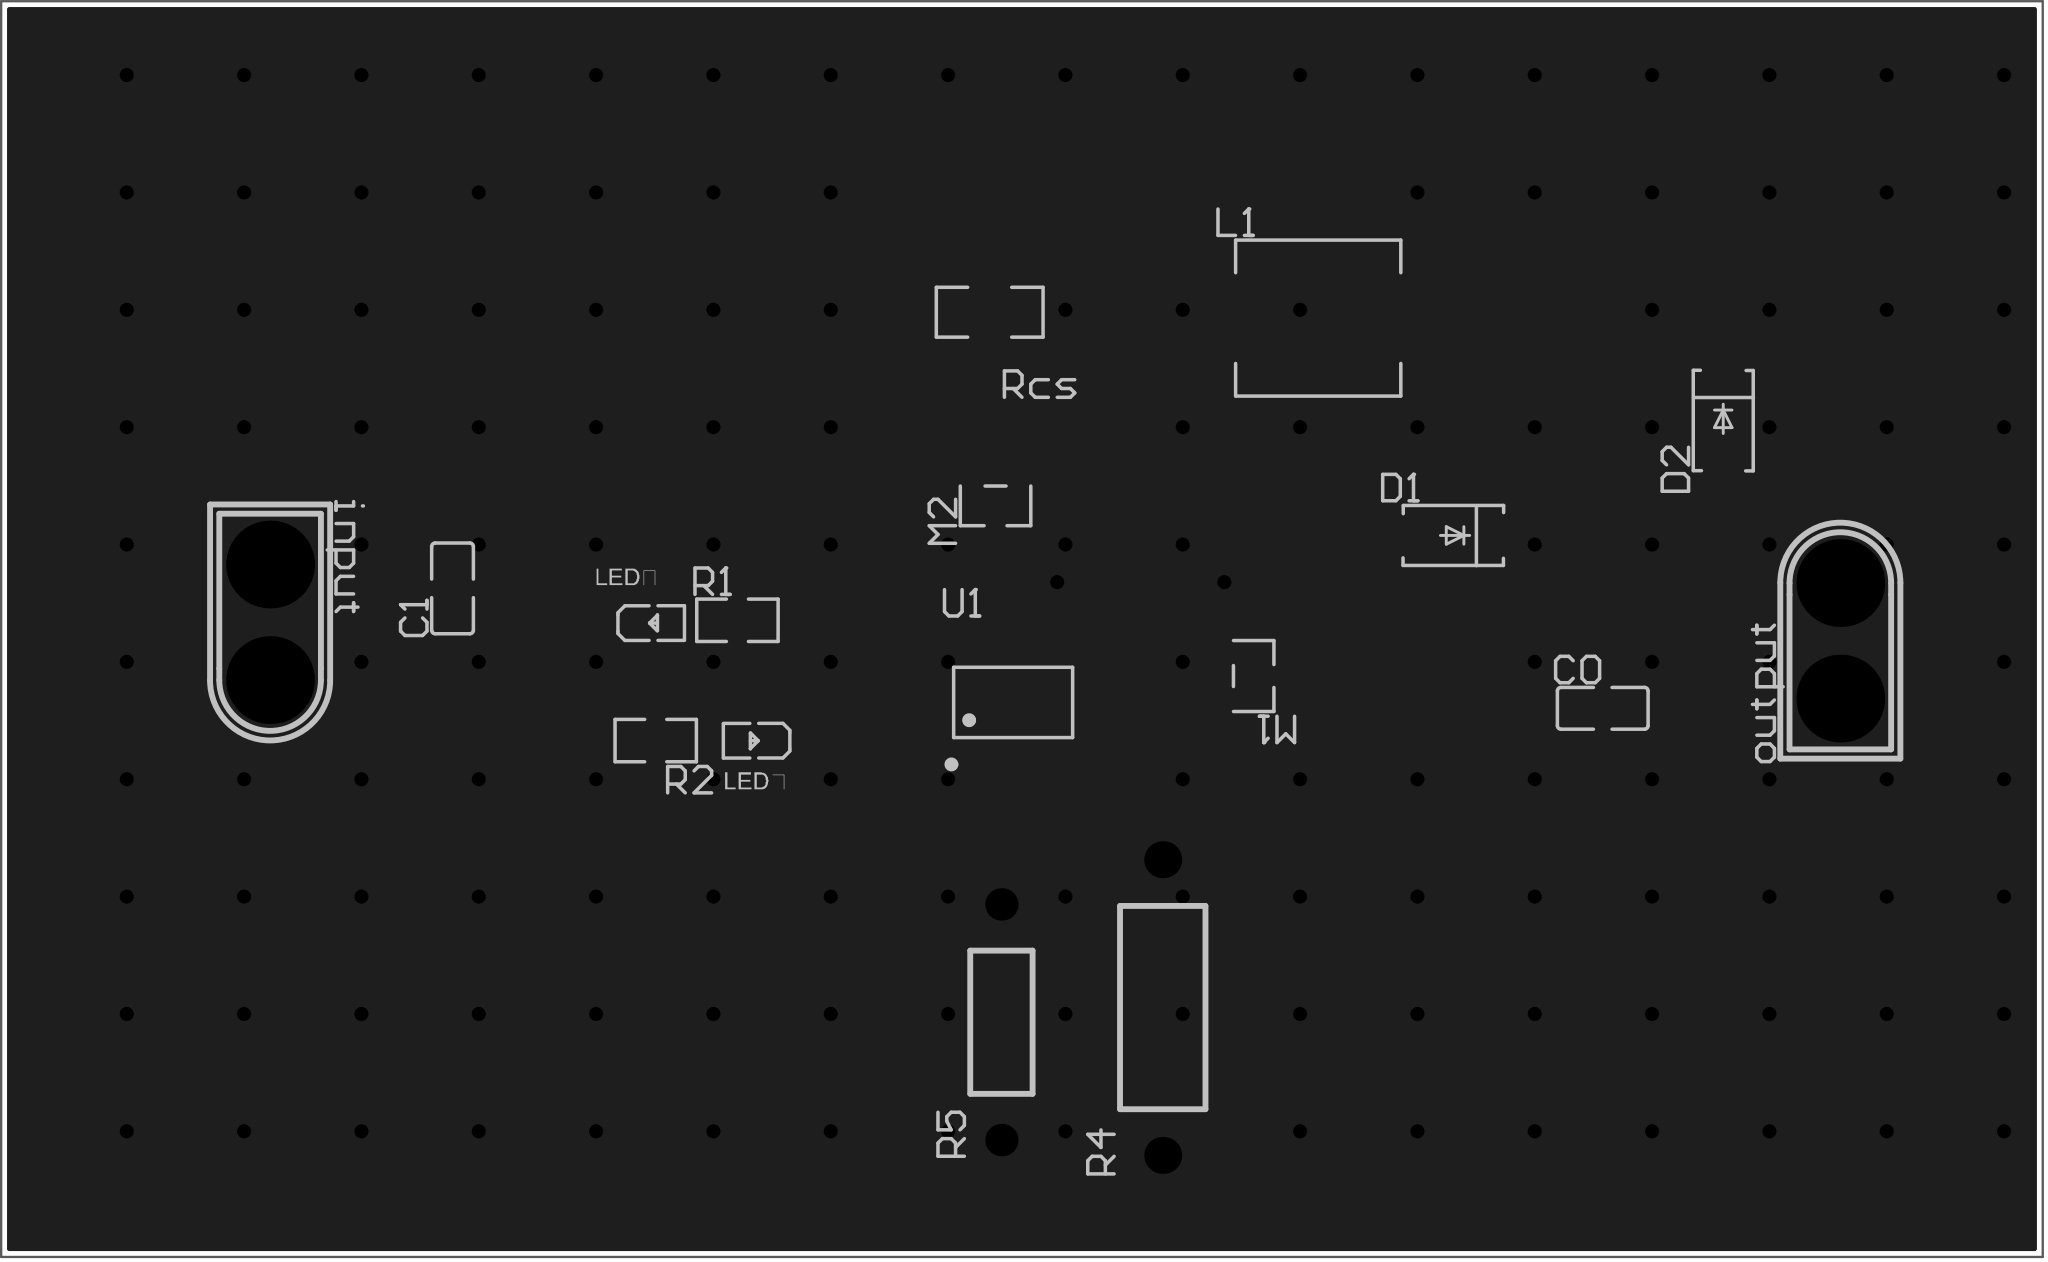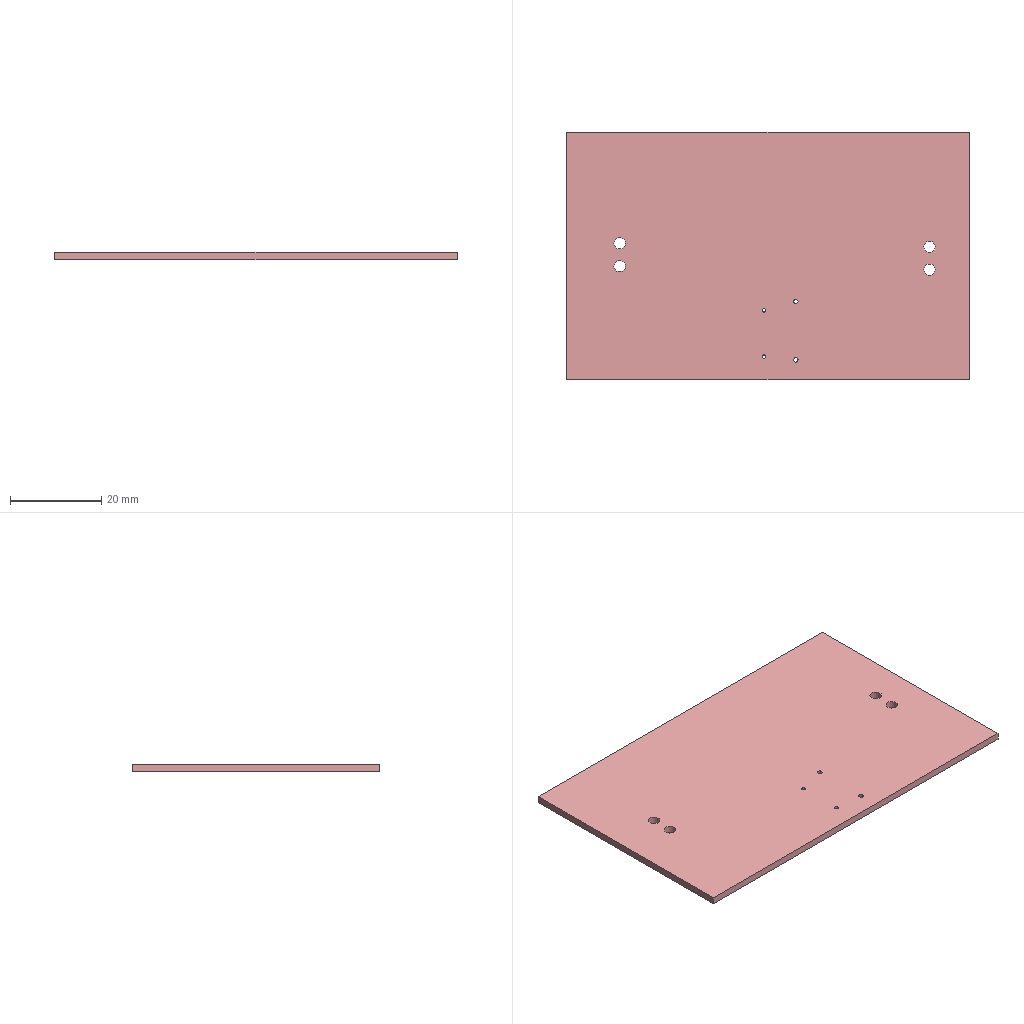Circuit board layout | Altium Designer | box 88.4 x 54.4 x 1.6 mm
Layer stack:
# Altium Designer layer stack of  (unit mm; dielectric type: 0 none, 1 core, 2 prepreg, 3 surface material)
index,name,kind,layer,copper_thickness_mm,dielectric_type,dielectric_thickness_mm,dielectric_material,dielectric_constant
0,Top Paste Mask Layer,other,,,,,,
1,Top Silkscreen Layer,other,,,,,,
2,Top Solder Mask Layer,dielectric,,,3,0.01,,3.3
3,Top Layer,copper,Top Layer,0.035,,,,
4,Dielectric1,dielectric,,,3,1.51,FR4,4.5
5,Bottom Layer,copper,Bottom Layer,0.035,,,,
6,Bottom Solder Mask Layer,dielectric,,,3,0.01,,3.3
7,Bottom Silkscreen Layer,other,,,,,,
8,Bottom Paste Mask Layer,other,,,,,,
# drill layer pairs: low layer,high layer
drill_pair,Top Layer,Bottom Layer
Part placement:
Designator,Comment,Layer,Footprint,Center-X(mm),Center-Y(mm),Rotation
C0,10uF,TopLayer,C0805,149.733,102.235,0
C1,10uF,TopLayer,C0805,99.933,107.426,90
D1,SS24,TopLayer,SMA_L4.3-W2.6-LS5.0-FD,143.256,109.728,0
D2,SS24,TopLayer,SMA_L4.3-W2.6-LS5.0-FD,154.94,114.681,90
input,XT30U-M,TopLayer,CONN-TH_XT30U-M,92.035,105.958,270
L1,22uH,TopLayer,IND-SMD_L7.0-W6.6_FXL0630,137.414,119.126,0
LED红,NCD0603Y2,TopLayer,LED0603-RD,113.049,100.838,180
LED绿,NCD0603Y2,TopLayer,LED0603-RD,108.585,105.918,0
M1,SI2300DS-T1-GE3,TopLayer,SOT-23-3_L2.9-W1.6-P1.90-LS2.8-BR,134.62,103.632,180
M2,SI2301CDS-T1-GE3,TopLayer,SOT-23-3_L3.0-W1.7-P0.95-LS2.9-BR,123.444,110.998,90
output,XT30U-M,TopLayer,CONN-TH_XT30U-M,160.02,105.156,90
R1,10kΩ,TopLayer,R0805,112.268,106.045,0
R2,10kΩ,TopLayer,R0805,108.731,100.838,180
R4,600kΩ,TopLayer,RES-TH_BD3.7-L8.7-P12.8-D0.8,130.683,89.281,90
R5,100kΩ,TopLayer,RES-TH_BD2.7-L6.2-P10.20-D0.4,123.698,88.646,90
Rcs,150mΩ,TopLayer,R1206,123.19,119.38,180
U1,CN3305,TopLayer,SOP-8_L4.9-W3.9-P1.27-LS6.0-BL-1,124.206,102.489,0
Pad and via stacks:
# Altium Designer via and pad stacks of  (unit mm). Each distinct definition once, with the count of objects using it.
# via: kind,start_layer,end_layer,hole_mm,diameter_mm,mode(0 simple;1 top-mid-bottom;2 full stack),diameter_per_layer,count,example_net
# pad: kind,layer,hole_mm,hole_type(0 round;1 square;2 slot),plating,top_size,top_shape(1 round;2 rect;3 octagon;9 rounded rect),mid_size,bottom_size,mode,footprint,size_per_layer,count,example
pad,Top Layer,0,0,plated,1.41x1.35,2,1.41x1.35,1.41x1.35,0,C0805,,3,C0.2
pad,Top Layer,0,0,plated,1.27x1.27,2,1.27x1.27,1.27x1.27,0,C0805,,1,C1.2
pad,Top Layer,0,0,plated,1.8x1.62,2,1.8x1.62,1.8x1.62,0,SMA_L4.3-W2.6-LS5.0-FD,,4,D1.1
pad,Top Layer,0,0,plated,2.424x3.62,2,2.424x3.62,2.424x3.62,0,IND-SMD_L7.0-W6.6_FXL0630,,2,L1.1
pad,Top Layer,0,0,plated,0.8x0.8,2,0.8x0.8,0.8x0.8,0,LED0603-RD,,4,LED\u7EA2.2
pad,Top Layer,0,0,plated,1.07x0.6,2,1.07x0.6,1.07x0.6,0,SOT-23-3_L2.9-W1.6-P1.90-LS2.8-BR,,3,M1.1
pad,Top Layer,0,0,plated,1.038x0.532,2,1.038x0.532,1.038x0.532,0,SOT-23-3_L3.0-W1.7-P0.95-LS2.9-BR,,3,M2.1
pad,Top Layer,0,0,plated,1.133x1.377,2,1.133x1.377,1.133x1.377,0,R0805,,4,R1.2
pad,Top Layer,0,0,plated,1.208x1.701,2,1.208x1.701,1.208x1.701,0,R1206,,2,Rcs.2
pad,Top Layer,0,0,plated,0.63x1.865,1,0.63x1.865,0.63x1.865,0,SOP-8_L4.9-W3.9-P1.27-LS6.0-BL-1,,8,U1.5
pad,Multi-Layer,2.54,0,plated,3.8x3.8,1,3.8x3.8,3.8x3.8,0,CONN-TH_XT30U-M,,4,input.1
pad,Multi-Layer,1,0,plated,1.6x1.6,1,1.6x1.6,1.6x1.6,0,RES-TH_BD3.7-L8.7-P12.8-D0.8,,2,R4.2
pad,Multi-Layer,0.8,0,plated,1.4x1.4,1,1.4x1.4,1.4x1.4,0,RES-TH_BD2.7-L6.2-P10.20-D0.4,,2,R5.1
via,Top Layer,Bottom Layer,0.3048,0.61,0,,153,$1N6
Copper pours:
name,layer,net,type(0 solid;1 hatched;2 none)
Top Layer-GND,Top Layer,GND,0
Bottom Layer-GND,Bottom Layer,GND,0